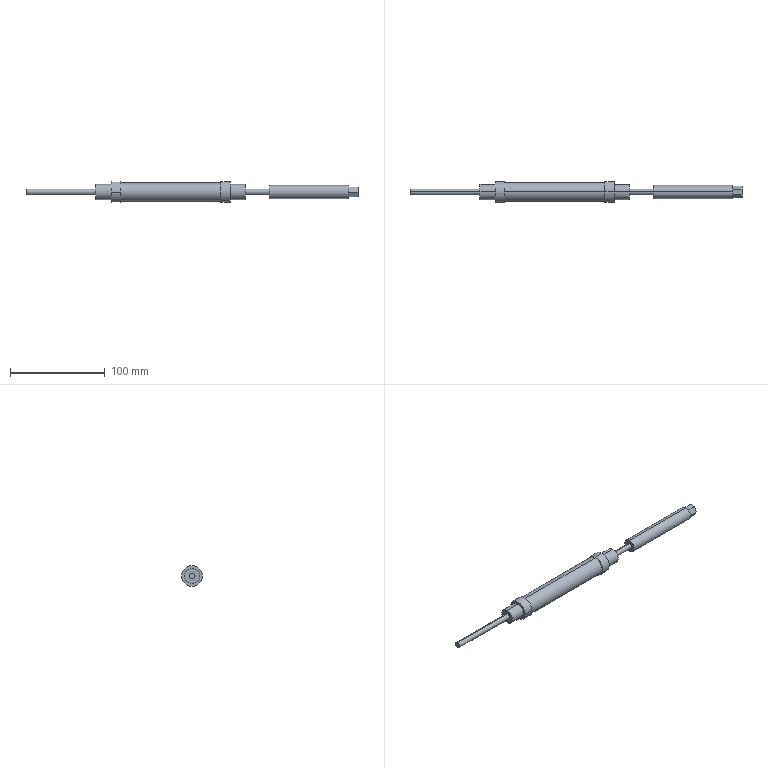Part | STEP file | Cylinder MALJ 16×75-40-S Extend | 2 solids | 30 faces | box 351 x 22 x 22 mm | volume 68468 mm3 | plane 16 | cylinder 14 | commonest cylinder face diameters 16 x4 22 x4 6 x2 14 x2 20 x2